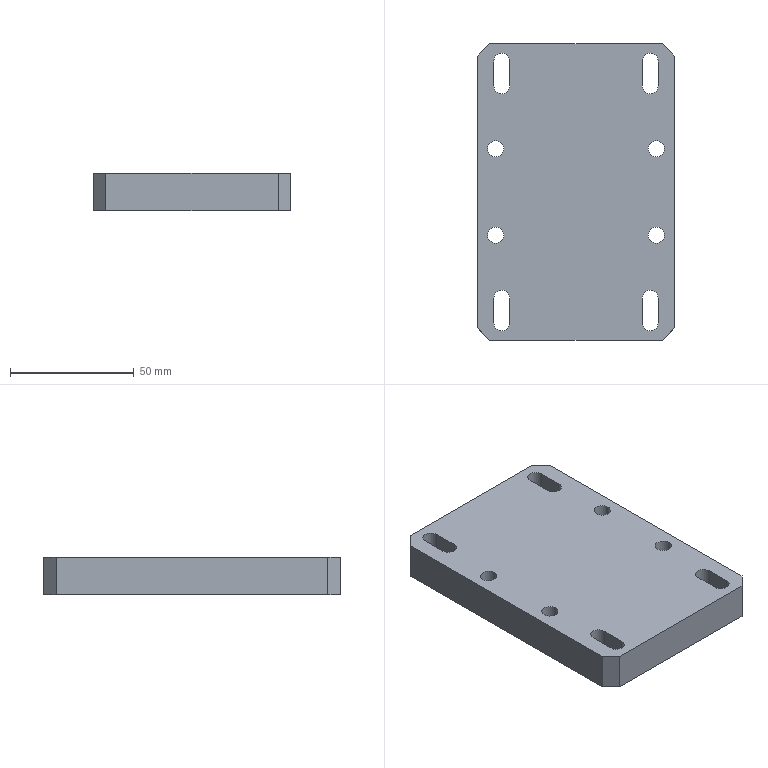Part | STEP file | PN_0013 | 1 solid | 54 faces | box 80 x 120 x 15 mm | volume 132965 mm3 | cylinder 28 | plane 22 | cone 4 | commonest cylinder face diameters 6.5 x8 6.6 x8 11 x8 5 x4